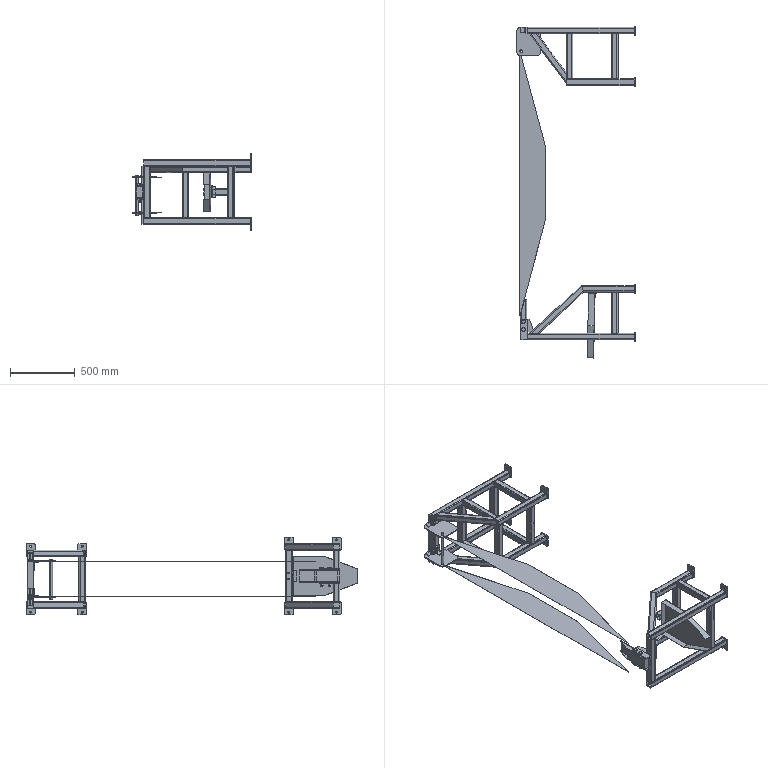Part | SolidWorks | features MirrorCompFeat 1, ReferencePattern 1 | 57 solids | 934 faces | box 917 x 2571 x 600 mm | volume 11540187 mm3 | plane 519 | cylinder 393 | cone 10 | spline 8 | torus 4 | commonest cylinder face diameters 8 x116 16 x112 20 x50 14 x21 10.5 x15 12.5 x15